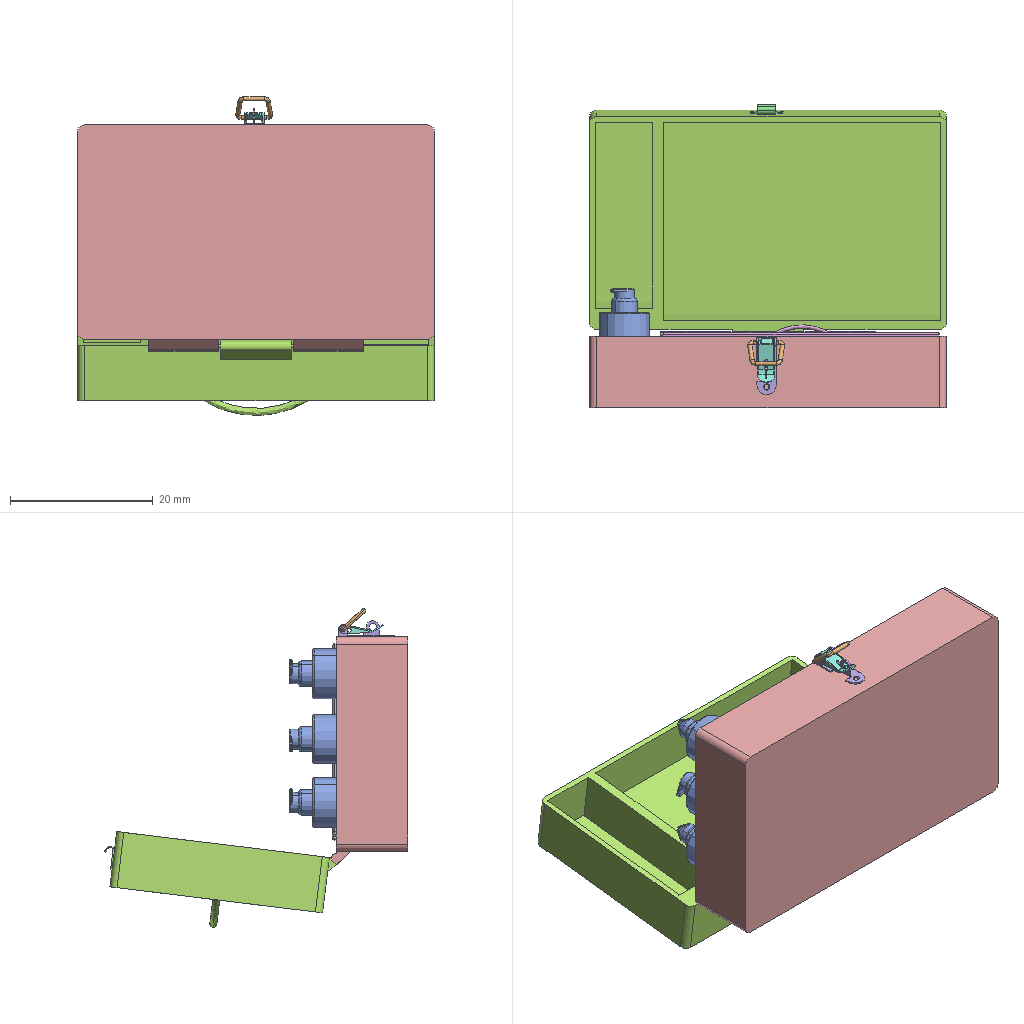Assembly | SolidWorks | 8 different items | 10 placed | box 50 x 43 x 45 mm
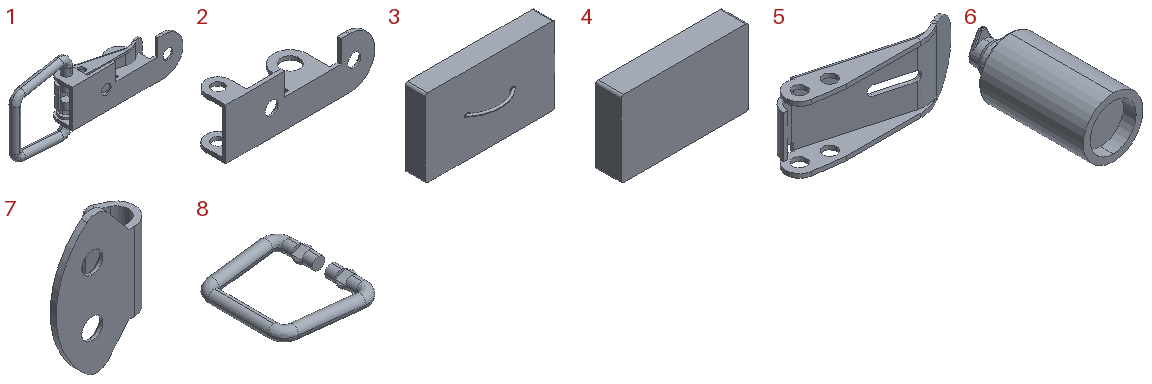Parts list (item | name | quantity | parent item | size | volume | features):
1 | (subassembly) | x1 | - | 11.513 x 2.3 x 5.2 mm | 11.366 mm3 | -
2 | - | x1 | in 1 | 7.94 x 2.3 x 2.72 mm | 4.422 mm3 | features BaseBody 1, Scale 1
3 | - | x1 | - | 50 x 12.396 x 31.7 mm | 2667 mm3 | features Fillet 2, ICE 2, BossThin 1, Extrusion 1, Shell 1, Sweep 1
4 | - | x1 | - | 50 x 10.7 x 31.711 mm | 5162 mm3 | features ICE 17, Stock 4, CirPattern 3, MoveCopyBody 3, Extrusion 1, Fillet 1, Shell 1
5 | - | x1 | in 1 | 6.154 x 1.321 x 2.4 mm | 2.823 mm3 | features BaseBody 1, Scale 1
6 | - | x3 | - | 7 x 15.6 x 7 mm | 176.298 mm3 | features ICE 5, Fillet 3, Shell 2, Extrusion 1
7 | - | x1 | - | 3.2 x 1.4 x 4.6 mm | 2.668 mm3 | features BaseBody 1, Scale 1
8 | - | x1 | in 1 | 4.596 x 5.2 x 0.6 mm | 4.12 mm3 | features BaseBody 1, Scale 1
Mates (type | each side: item.copy, entity, surface, feature):
In the top assembly
Concentric | 4.1 face cylinder Boss-Extrude21 | 3.1 face cylinder Boss-Extrude2
Coincident | 4.1 face plane Boss-Extrude2 | 3.1 face plane Boss-Extrude1
Concentric | 4.1 face cylinder Boss-Extrude12 | 6.1 face cylinder Shell1
Coincident | 4.1 face plane Boss-Extrude12 | 6.1 face plane Shell1
Concentric | 4.1 face cylinder CirPattern5 | 6.2 face cylinder Boss-Extrude1
Concentric | 4.1 face cylinder CirPattern6 | 6.3 face cylinder Boss-Extrude1
Coincident | 4.1 face plane Boss-Extrude13 | 6.2 face plane Shell1
Coincident | 4.1 face plane Boss-Extrude14 | 6.3 face plane Shell1
Coincident | 3.1 face plane Boss-Extrude1 | 7.1 face plane Input1
Parallel | 3.1 face plane Boss-Extrude1 | 7.1 face plane Input1
Coincident | 4.1 face plane Boss-Extrude2 | 2.1 face plane Input1
Parallel | 4.1 face plane Boss-Extrude2 | 5.1 face plane Input1
Lock | 3.1 select_type:0 | 7.1 select_type:0
Lock | 4.1 select_type:0 | 2.1 select_type:0
In subassembly 1
Concentric | 8.1 face cylinder Input1 | 2.2 face cylinder Input1
Coincident | 8.1 face plane Input1 | 2.2 face plane Input1
Concentric | 5.2 face cylinder Input1 | 8.1 face cylinder Input1
DistanceDim | 2.2 face plane Input1 | 5.2 face plane Input1